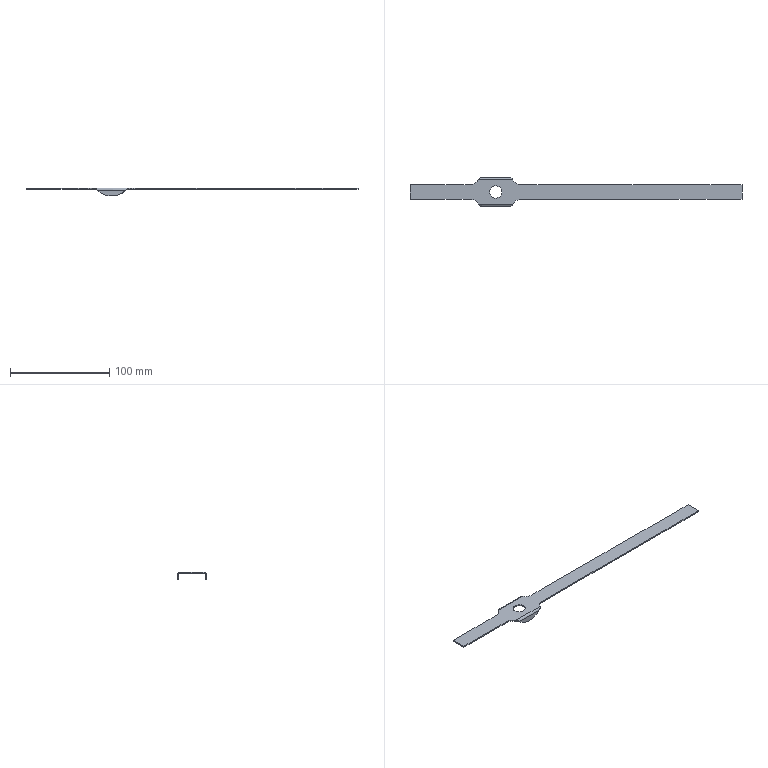Part | STEP file | gslz 2016.10.28-13_id1142_x_t | 1 solid | 32 faces | box 335 x 29 x 8 mm | volume 7083 mm3 | plane 12 | other 11 | cylinder 5 | spline 4 | commonest cylinder face diameters 1.5 x2 4 x2 12.3 x1